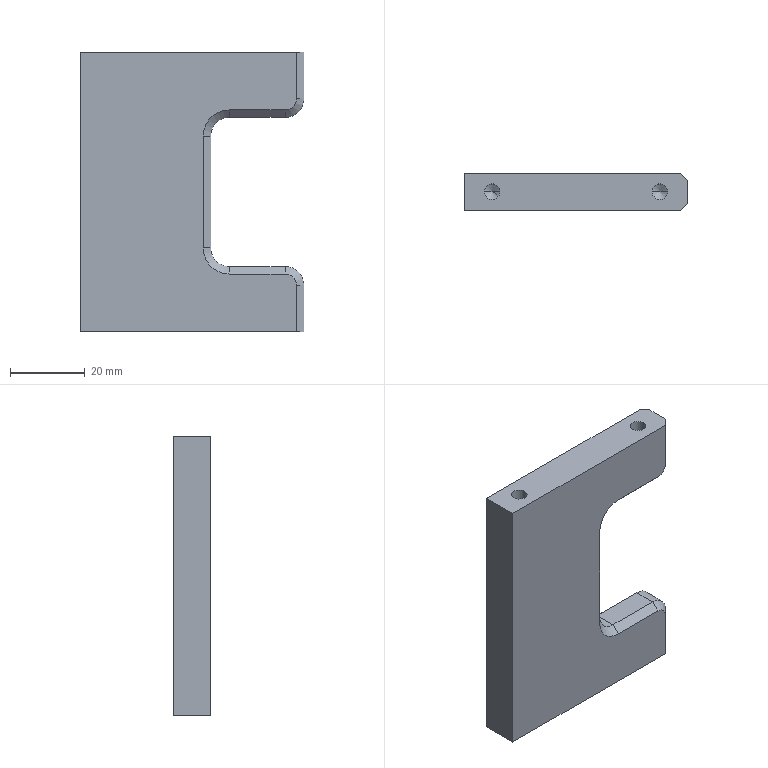Part | SolidWorks | features HoleWzd 2, Chamfer 1, Extrusion 1, Fillet 1, ICE 1 | 1 solid | 48 faces | box 60 x 10 x 75 mm | volume 33824 mm3 | plane 20 | cone 16 | cylinder 12 | commonest cylinder face diameters 4.2 x8 10 x4
STEP:
#1=CARTESIAN_POINT('',(50.4,5.,-12.4));
#2=VERTEX_POINT('',#1);
#3=CARTESIAN_POINT('',(54.6,5.,-12.4));
#4=VERTEX_POINT('',#3);
#5=CARTESIAN_POINT('',(52.5,5.,-12.4));
#6=DIRECTION('',(0.,0.,1.));
#7=DIRECTION('',(1.,0.,0.));
#8=AXIS2_PLACEMENT_3D('',#5,#6,#7);
#9=CIRCLE('',#8,2.1);
#10=EDGE_CURVE('',#2,#4,#9,.T.);
#11=ORIENTED_EDGE('',*,*,#10,.F.);
#12=CARTESIAN_POINT('',(50.4,5.,0.));
#13=VERTEX_POINT('',#12);
#14=CARTESIAN_POINT('',(50.4,5.,0.));
#15=DIRECTION('',(0.,0.,1.));
#16=VECTOR('',#15,1000.);
#17=LINE('',#14,#16);
#18=EDGE_CURVE('',#2,#13,#17,.T.);
#19=ORIENTED_EDGE('',*,*,#18,.T.);
#20=CARTESIAN_POINT('',(54.6,5.,0.));
#21=VERTEX_POINT('',#20);
#22=CARTESIAN_POINT('',(52.5,5.,0.));
#23=DIRECTION('',(0.,0.,1.));
#24=DIRECTION('',(1.,0.,0.));
#25=AXIS2_PLACEMENT_3D('',#22,#23,#24);
#26=CIRCLE('',#25,2.1);
#27=EDGE_CURVE('',#13,#21,#26,.T.);
#28=ORIENTED_EDGE('',*,*,#27,.T.);
#29=CARTESIAN_POINT('',(54.6,5.,0.));
#30=DIRECTION('',(0.,0.,1.));
#31=VECTOR('',#30,1000.);
#32=LINE('',#29,#31);
#33=EDGE_CURVE('',#4,#21,#32,.T.);
#34=ORIENTED_EDGE('',*,*,#33,.F.);
#35=EDGE_LOOP('',(#11,#19,#28,#34));
#36=FACE_OUTER_BOUND('',#35,.T.);
#37=CARTESIAN_POINT('',(52.5,5.,0.));
#38=DIRECTION('',(0.,0.,1.));
#39=DIRECTION('',(1.,0.,0.));
#40=AXIS2_PLACEMENT_3D('',#37,#38,#39);
#41=CYLINDRICAL_SURFACE('',#40,2.1);
#42=ADVANCED_FACE('',(#36),#41,.F.);
#43=CARTESIAN_POINT('',(52.5,5.,-13.662));
#44=VERTEX_POINT('',#43);
#45=CARTESIAN_POINT('',(54.6,5.,-12.4));
#46=DIRECTION('',(0.8572,0.,0.515));
#47=VECTOR('',#46,1000.);
#48=LINE('',#45,#47);
#49=EDGE_CURVE('',#44,#4,#48,.T.);
#50=ORIENTED_EDGE('',*,*,#49,.F.);
#51=CARTESIAN_POINT('',(50.4,5.,-12.4));
#52=DIRECTION('',(-0.8572,0.,0.515));
#53=VECTOR('',#52,1000.);
#54=LINE('',#51,#53);
#55=EDGE_CURVE('',#44,#2,#54,.T.);
#56=ORIENTED_EDGE('',*,*,#55,.T.);
#57=ORIENTED_EDGE('',*,*,#10,.T.);
#58=EDGE_LOOP('',(#50,#56,#57));
#59=FACE_OUTER_BOUND('',#58,.T.);
#60=CARTESIAN_POINT('',(52.5,5.,-12.4));
#61=DIRECTION('',(0.,0.,1.));
#62=DIRECTION('',(1.,0.,0.));
#63=AXIS2_PLACEMENT_3D('',#60,#61,#62);
#64=CONICAL_SURFACE('',#63,2.1,1.03);
#65=ADVANCED_FACE('',(#59),#64,.F.);
#66=CARTESIAN_POINT('',(5.4,5.,-12.4));
#67=VERTEX_POINT('',#66);
#68=CARTESIAN_POINT('',(9.6,5.,-12.4));
#69=VERTEX_POINT('',#68);
#70=CARTESIAN_POINT('',(7.5,5.,-12.4));
#71=DIRECTION('',(0.,0.,1.));
#72=DIRECTION('',(1.,0.,0.));
#73=AXIS2_PLACEMENT_3D('',#70,#71,#72);
#74=CIRCLE('',#73,2.1);
#75=EDGE_CURVE('',#67,#69,#74,.T.);
#76=ORIENTED_EDGE('',*,*,#75,.F.);
#77=CARTESIAN_POINT('',(5.4,5.,0.));
#78=VERTEX_POINT('',#77);
#79=CARTESIAN_POINT('',(5.4,5.,0.));
#80=DIRECTION('',(0.,0.,1.));
#81=VECTOR('',#80,1000.);
#82=LINE('',#79,#81);
#83=EDGE_CURVE('',#67,#78,#82,.T.);
#84=ORIENTED_EDGE('',*,*,#83,.T.);
#85=CARTESIAN_POINT('',(9.6,5.,0.));
#86=VERTEX_POINT('',#85);
#87=CARTESIAN_POINT('',(7.5,5.,0.));
#88=DIRECTION('',(0.,0.,1.));
#89=DIRECTION('',(1.,0.,0.));
#90=AXIS2_PLACEMENT_3D('',#87,#88,#89);
#91=CIRCLE('',#90,2.1);
#92=EDGE_CURVE('',#78,#86,#91,.T.);
#93=ORIENTED_EDGE('',*,*,#92,.T.);
#94=CARTESIAN_POINT('',(9.6,5.,0.));
#95=DIRECTION('',(0.,0.,1.));
#96=VECTOR('',#95,1000.);
#97=LINE('',#94,#96);
#98=EDGE_CURVE('',#69,#86,#97,.T.);
#99=ORIENTED_EDGE('',*,*,#98,.F.);
#100=EDGE_LOOP('',(#76,#84,#93,#99));
#101=FACE_OUTER_BOUND('',#100,.T.);
#102=CARTESIAN_POINT('',(7.5,5.,0.));
#103=DIRECTION('',(0.,0.,1.));
#104=DIRECTION('',(1.,0.,0.));
#105=AXIS2_PLACEMENT_3D('',#102,#103,#104);
#106=CYLINDRICAL_SURFACE('',#105,2.1);
#107=ADVANCED_FACE('',(#101),#106,.F.);
#108=CARTESIAN_POINT('',(7.5,5.,-13.662));
#109=VERTEX_POINT('',#108);
#110=CARTESIAN_POINT('',(9.6,5.,-12.4));
#111=DIRECTION('',(0.8572,0.,0.515));
#112=VECTOR('',#111,1000.);
#113=LINE('',#110,#112);
#114=EDGE_CURVE('',#109,#69,#113,.T.);
#115=ORIENTED_EDGE('',*,*,#114,.F.);
#116=CARTESIAN_POINT('',(5.4,5.,-12.4));
#117=DIRECTION('',(-0.8572,0.,0.515));
#118=VECTOR('',#117,1000.);
#119=LINE('',#116,#118);
#120=EDGE_CURVE('',#109,#67,#119,.T.);
#121=ORIENTED_EDGE('',*,*,#120,.T.);
#122=ORIENTED_EDGE('',*,*,#75,.T.);
#123=EDGE_LOOP('',(#115,#121,#122));
#124=FACE_OUTER_BOUND('',#123,.T.);
#125=CARTESIAN_POINT('',(7.5,5.,-12.4));
#126=DIRECTION('',(0.,0.,1.));
#127=DIRECTION('',(1.,0.,0.));
#128=AXIS2_PLACEMENT_3D('',#125,#126,#127);
#129=CONICAL_SURFACE('',#128,2.1,1.03);
#130=ADVANCED_FACE('',(#124),#129,.F.);
#131=CARTESIAN_POINT('',(9.6,5.,-62.6));
#132=VERTEX_POINT('',#131);
#133=CARTESIAN_POINT('',(5.4,5.,-62.6));
#134=VERTEX_POINT('',#133);
#135=CARTESIAN_POINT('',(7.5,5.,-62.6));
#136=DIRECTION('',(0.,0.,-1.));
#137=DIRECTION('',(-1.,0.,0.));
#138=AXIS2_PLACEMENT_3D('',#135,#136,#137);
#139=CIRCLE('',#138,2.1);
#140=EDGE_CURVE('',#132,#134,#139,.T.);
#141=ORIENTED_EDGE('',*,*,#140,.F.);
#142=CARTESIAN_POINT('',(9.6,5.,-75.));
#143=VERTEX_POINT('',#142);
#144=CARTESIAN_POINT('',(9.6,5.,-75.));
#145=DIRECTION('',(0.,0.,-1.));
#146=VECTOR('',#145,1000.);
#147=LINE('',#144,#146);
#148=EDGE_CURVE('',#132,#143,#147,.T.);
#149=ORIENTED_EDGE('',*,*,#148,.T.);
#150=CARTESIAN_POINT('',(5.4,5.,-75.));
#151=VERTEX_POINT('',#150);
#152=CARTESIAN_POINT('',(7.5,5.,-75.));
#153=DIRECTION('',(0.,0.,-1.));
#154=DIRECTION('',(-1.,0.,0.));
#155=AXIS2_PLACEMENT_3D('',#152,#153,#154);
#156=CIRCLE('',#155,2.1);
#157=EDGE_CURVE('',#143,#151,#156,.T.);
#158=ORIENTED_EDGE('',*,*,#157,.T.);
#159=CARTESIAN_POINT('',(5.4,5.,-75.));
#160=DIRECTION('',(0.,0.,-1.));
#161=VECTOR('',#160,1000.);
#162=LINE('',#159,#161);
#163=EDGE_CURVE('',#134,#151,#162,.T.);
#164=ORIENTED_EDGE('',*,*,#163,.F.);
#165=EDGE_LOOP('',(#141,#149,#158,#164));
#166=FACE_OUTER_BOUND('',#165,.T.);
#167=CARTESIAN_POINT('',(7.5,5.,-75.));
#168=DIRECTION('',(0.,0.,-1.));
#169=DIRECTION('',(-1.,0.,0.));
#170=AXIS2_PLACEMENT_3D('',#167,#168,#169);
#171=CYLINDRICAL_SURFACE('',#170,2.1);
#172=ADVANCED_FACE('',(#166),#171,.F.);
#173=CARTESIAN_POINT('',(7.5,5.,-61.338));
#174=VERTEX_POINT('',#173);
#175=CARTESIAN_POINT('',(5.4,5.,-62.6));
#176=DIRECTION('',(-0.8572,0.,-0.515));
#177=VECTOR('',#176,1000.);
#178=LINE('',#175,#177);
#179=EDGE_CURVE('',#174,#134,#178,.T.);
#180=ORIENTED_EDGE('',*,*,#179,.F.);
#181=CARTESIAN_POINT('',(9.6,5.,-62.6));
#182=DIRECTION('',(0.8572,0.,-0.515));
#183=VECTOR('',#182,1000.);
#184=LINE('',#181,#183);
#185=EDGE_CURVE('',#174,#132,#184,.T.);
#186=ORIENTED_EDGE('',*,*,#185,.T.);
#187=ORIENTED_EDGE('',*,*,#140,.T.);
#188=EDGE_LOOP('',(#180,#186,#187));
#189=FACE_OUTER_BOUND('',#188,.T.);
#190=CARTESIAN_POINT('',(7.5,5.,-62.6));
#191=DIRECTION('',(0.,0.,-1.));
#192=DIRECTION('',(-1.,0.,0.));
#193=AXIS2_PLACEMENT_3D('',#190,#191,#192);
#194=CONICAL_SURFACE('',#193,2.1,1.03);
#195=ADVANCED_FACE('',(#189),#194,.F.);
#196=CARTESIAN_POINT('',(54.6,5.,-62.6));
#197=VERTEX_POINT('',#196);
#198=CARTESIAN_POINT('',(50.4,5.,-62.6));
#199=VERTEX_POINT('',#198);
#200=CARTESIAN_POINT('',(52.5,5.,-62.6));
#201=DIRECTION('',(0.,0.,-1.));
#202=DIRECTION('',(-1.,0.,0.));
#203=AXIS2_PLACEMENT_3D('',#200,#201,#202);
#204=CIRCLE('',#203,2.1);
#205=EDGE_CURVE('',#197,#199,#204,.T.);
#206=ORIENTED_EDGE('',*,*,#205,.F.);
#207=CARTESIAN_POINT('',(54.6,5.,-75.));
#208=VERTEX_POINT('',#207);
#209=CARTESIAN_POINT('',(54.6,5.,-75.));
#210=DIRECTION('',(0.,0.,-1.));
#211=VECTOR('',#210,1000.);
#212=LINE('',#209,#211);
#213=EDGE_CURVE('',#197,#208,#212,.T.);
#214=ORIENTED_EDGE('',*,*,#213,.T.);
#215=CARTESIAN_POINT('',(50.4,5.,-75.));
#216=VERTEX_POINT('',#215);
#217=CARTESIAN_POINT('',(52.5,5.,-75.));
#218=DIRECTION('',(0.,0.,-1.));
#219=DIRECTION('',(-1.,0.,0.));
#220=AXIS2_PLACEMENT_3D('',#217,#218,#219);
#221=CIRCLE('',#220,2.1);
#222=EDGE_CURVE('',#208,#216,#221,.T.);
#223=ORIENTED_EDGE('',*,*,#222,.T.);
#224=CARTESIAN_POINT('',(50.4,5.,-75.));
#225=DIRECTION('',(0.,0.,-1.));
#226=VECTOR('',#225,1000.);
#227=LINE('',#224,#226);
#228=EDGE_CURVE('',#199,#216,#227,.T.);
#229=ORIENTED_EDGE('',*,*,#228,.F.);
#230=EDGE_LOOP('',(#206,#214,#223,#229));
#231=FACE_OUTER_BOUND('',#230,.T.);
#232=CARTESIAN_POINT('',(52.5,5.,-75.));
#233=DIRECTION('',(0.,0.,-1.));
#234=DIRECTION('',(-1.,0.,0.));
#235=AXIS2_PLACEMENT_3D('',#232,#233,#234);
#236=CYLINDRICAL_SURFACE('',#235,2.1);
#237=ADVANCED_FACE('',(#231),#236,.F.);
#238=CARTESIAN_POINT('',(52.5,5.,-61.338));
#239=VERTEX_POINT('',#238);
#240=CARTESIAN_POINT('',(50.4,5.,-62.6));
#241=DIRECTION('',(-0.8572,0.,-0.515));
#242=VECTOR('',#241,1000.);
#243=LINE('',#240,#242);
#244=EDGE_CURVE('',#239,#199,#243,.T.);
#245=ORIENTED_EDGE('',*,*,#244,.F.);
#246=CARTESIAN_POINT('',(54.6,5.,-62.6));
#247=DIRECTION('',(0.8572,0.,-0.515));
#248=VECTOR('',#247,1000.);
#249=LINE('',#246,#248);
#250=EDGE_CURVE('',#239,#197,#249,.T.);
#251=ORIENTED_EDGE('',*,*,#250,.T.);
#252=ORIENTED_EDGE('',*,*,#205,.T.);
#253=EDGE_LOOP('',(#245,#251,#252));
#254=FACE_OUTER_BOUND('',#253,.T.);
#255=CARTESIAN_POINT('',(52.5,5.,-62.6));
#256=DIRECTION('',(0.,0.,-1.));
#257=DIRECTION('',(-1.,0.,0.));
#258=AXIS2_PLACEMENT_3D('',#255,#256,#257);
#259=CONICAL_SURFACE('',#258,2.1,1.03);
#260=ADVANCED_FACE('',(#254),#259,.F.);
#261=CARTESIAN_POINT('',(60.,8.,-62.5));
#262=VERTEX_POINT('',#261);
#263=CARTESIAN_POINT('',(60.,2.,-62.5));
#264=VERTEX_POINT('',#263);
#265=CARTESIAN_POINT('',(60.,10.,-62.5));
#266=DIRECTION('',(0.,-1.,0.));
#267=VECTOR('',#266,1000.);
#268=LINE('',#265,#267);
#269=EDGE_CURVE('',#262,#264,#268,.T.);
#270=ORIENTED_EDGE('',*,*,#269,.T.);
#271=CARTESIAN_POINT('',(60.,2.,-75.));
#272=VERTEX_POINT('',#271);
#273=CARTESIAN_POINT('',(60.,2.,-75.));
#274=DIRECTION('',(0.,0.,-1.));
#275=VECTOR('',#274,1000.);
#276=LINE('',#273,#275);
#277=EDGE_CURVE('',#264,#272,#276,.T.);
#278=ORIENTED_EDGE('',*,*,#277,.T.);
#279=CARTESIAN_POINT('',(60.,8.,-75.));
#280=VERTEX_POINT('',#279);
#281=CARTESIAN_POINT('',(60.,10.,-75.));
#282=DIRECTION('',(0.,-1.,0.));
#283=VECTOR('',#282,1000.);
#284=LINE('',#281,#283);
#285=EDGE_CURVE('',#280,#272,#284,.T.);
#286=ORIENTED_EDGE('',*,*,#285,.F.);
#287=CARTESIAN_POINT('',(60.,8.,0.));
#288=DIRECTION('',(0.,0.,1.));
#289=VECTOR('',#288,1000.);
#290=LINE('',#287,#289);
#291=EDGE_CURVE('',#280,#262,#290,.T.);
#292=ORIENTED_EDGE('',*,*,#291,.T.);
#293=EDGE_LOOP('',(#270,#278,#286,#292));
#294=FACE_OUTER_BOUND('',#293,.T.);
#295=CARTESIAN_POINT('',(60.,10.,0.));
#296=DIRECTION('',(-1.,0.,0.));
#297=DIRECTION('',(0.,0.,1.));
#298=AXIS2_PLACEMENT_3D('',#295,#296,#297);
#299=PLANE('',#298);
#300=ADVANCED_FACE('',(#294),#299,.F.);
#301=CARTESIAN_POINT('',(0.,0.,-75.));
#302=VERTEX_POINT('',#301);
#303=CARTESIAN_POINT('',(0.,0.,0.));
#304=VERTEX_POINT('',#303);
#305=CARTESIAN_POINT('',(0.,0.,0.));
#306=DIRECTION('',(0.,0.,1.));
#307=VECTOR('',#306,1000.);
#308=LINE('',#305,#307);
#309=EDGE_CURVE('',#302,#304,#308,.T.);
#310=ORIENTED_EDGE('',*,*,#309,.T.);
#311=CARTESIAN_POINT('',(0.,10.,0.));
#312=VERTEX_POINT('',#311);
#313=CARTESIAN_POINT('',(0.,10.,0.));
#314=DIRECTION('',(0.,-1.,0.));
#315=VECTOR('',#314,1000.);
#316=LINE('',#313,#315);
#317=EDGE_CURVE('',#312,#304,#316,.T.);
#318=ORIENTED_EDGE('',*,*,#317,.F.);
#319=CARTESIAN_POINT('',(0.,10.,-75.));
#320=VERTEX_POINT('',#319);
#321=CARTESIAN_POINT('',(0.,10.,0.));
#322=DIRECTION('',(0.,0.,1.));
#323=VECTOR('',#322,1000.);
#324=LINE('',#321,#323);
#325=EDGE_CURVE('',#320,#312,#324,.T.);
#326=ORIENTED_EDGE('',*,*,#325,.F.);
#327=CARTESIAN_POINT('',(0.,10.,-75.));
#328=DIRECTION('',(0.,-1.,0.));
#329=VECTOR('',#328,1000.);
#330=LINE('',#327,#329);
#331=EDGE_CURVE('',#320,#302,#330,.T.);
#332=ORIENTED_EDGE('',*,*,#331,.T.);
#333=EDGE_LOOP('',(#310,#318,#326,#332));
#334=FACE_OUTER_BOUND('',#333,.T.);
#335=CARTESIAN_POINT('',(0.,10.,0.));
#336=DIRECTION('',(1.,0.,0.));
#337=DIRECTION('',(0.,0.,-1.));
#338=AXIS2_PLACEMENT_3D('',#335,#336,#337);
#339=PLANE('',#338);
#340=ADVANCED_FACE('',(#334),#339,.F.);
#341=CARTESIAN_POINT('',(52.5,5.,0.));
#342=DIRECTION('',(0.,0.,1.));
#343=DIRECTION('',(1.,0.,0.));
#344=AXIS2_PLACEMENT_3D('',#341,#342,#343);
#345=CIRCLE('',#344,2.1);
#346=EDGE_CURVE('',#21,#13,#345,.T.);
#347=ORIENTED_EDGE('',*,*,#346,.F.);
#348=ORIENTED_EDGE('',*,*,#27,.F.);
#349=EDGE_LOOP('',(#347,#348));
#350=FACE_BOUND('',#349,.T.);
#351=CARTESIAN_POINT('',(7.5,5.,0.));
#352=DIRECTION('',(0.,0.,1.));
#353=DIRECTION('',(1.,0.,0.));
#354=AXIS2_PLACEMENT_3D('',#351,#352,#353);
#355=CIRCLE('',#354,2.1);
#356=EDGE_CURVE('',#86,#78,#355,.T.);
#357=ORIENTED_EDGE('',*,*,#356,.F.);
#358=ORIENTED_EDGE('',*,*,#92,.F.);
#359=EDGE_LOOP('',(#357,#358));
#360=FACE_BOUND('',#359,.T.);
#361=CARTESIAN_POINT('',(58.,0.,0.));
#362=VERTEX_POINT('',#361);
#363=CARTESIAN_POINT('',(0.,0.,0.));
#364=DIRECTION('',(1.,0.,0.));
#365=VECTOR('',#364,1000.);
#366=LINE('',#363,#365);
#367=EDGE_CURVE('',#304,#362,#366,.T.);
#368=ORIENTED_EDGE('',*,*,#367,.T.);
#369=CARTESIAN_POINT('',(60.,2.,0.));
#370=VERTEX_POINT('',#369);
#371=CARTESIAN_POINT('',(60.,2.,0.));
#372=DIRECTION('',(0.7071,0.7071,0.));
#373=VECTOR('',#372,1000.);
#374=LINE('',#371,#373);
#375=EDGE_CURVE('',#362,#370,#374,.T.);
#376=ORIENTED_EDGE('',*,*,#375,.T.);
#377=CARTESIAN_POINT('',(60.,8.,0.));
#378=VERTEX_POINT('',#377);
#379=CARTESIAN_POINT('',(60.,10.,0.));
#380=DIRECTION('',(0.,-1.,0.));
#381=VECTOR('',#380,1000.);
#382=LINE('',#379,#381);
#383=EDGE_CURVE('',#378,#370,#382,.T.);
#384=ORIENTED_EDGE('',*,*,#383,.F.);
#385=CARTESIAN_POINT('',(58.,10.,0.));
#386=VERTEX_POINT('',#385);
#387=CARTESIAN_POINT('',(58.,10.,0.));
#388=DIRECTION('',(-0.7071,0.7071,0.));
#389=VECTOR('',#388,1000.);
#390=LINE('',#387,#389);
#391=EDGE_CURVE('',#378,#386,#390,.T.);
#392=ORIENTED_EDGE('',*,*,#391,.T.);
#393=CARTESIAN_POINT('',(0.,10.,0.));
#394=DIRECTION('',(1.,0.,0.));
#395=VECTOR('',#394,1000.);
#396=LINE('',#393,#395);
#397=EDGE_CURVE('',#312,#386,#396,.T.);
#398=ORIENTED_EDGE('',*,*,#397,.F.);
#399=ORIENTED_EDGE('',*,*,#317,.T.);
#400=EDGE_LOOP('',(#368,#376,#384,#392,#398,#399));
#401=FACE_OUTER_BOUND('',#400,.T.);
#402=CARTESIAN_POINT('',(0.,10.,0.));
#403=DIRECTION('',(0.,0.,-1.));
#404=DIRECTION('',(-1.,0.,0.));
#405=AXIS2_PLACEMENT_3D('',#402,#403,#404);
#406=PLANE('',#405);
#407=ADVANCED_FACE('',(#350,#360,#401),#406,.F.);
#408=ORIENTED_EDGE('',*,*,#383,.T.);
#409=CARTESIAN_POINT('',(60.,2.,-12.5));
#410=VERTEX_POINT('',#409);
#411=CARTESIAN_POINT('',(60.,2.,-12.5));
#412=DIRECTION('',(0.,0.,-1.));
#413=VECTOR('',#412,1000.);
#414=LINE('',#411,#413);
#415=EDGE_CURVE('',#370,#410,#414,.T.);
#416=ORIENTED_EDGE('',*,*,#415,.T.);
#417=CARTESIAN_POINT('',(60.,8.,-12.5));
#418=VERTEX_POINT('',#417);
#419=CARTESIAN_POINT('',(60.,10.,-12.5));
#420=DIRECTION('',(0.,1.,0.));
#421=VECTOR('',#420,1000.);
#422=LINE('',#419,#421);
#423=EDGE_CURVE('',#410,#418,#422,.T.);
#424=ORIENTED_EDGE('',*,*,#423,.T.);
#425=CARTESIAN_POINT('',(60.,8.,0.));
#426=DIRECTION('',(0.,0.,1.));
#427=VECTOR('',#426,1000.);
#428=LINE('',#425,#427);
#429=EDGE_CURVE('',#418,#378,#428,.T.);
#430=ORIENTED_EDGE('',*,*,#429,.T.);
#431=EDGE_LOOP('',(#408,#416,#424,#430));
#432=FACE_OUTER_BOUND('',#431,.T.);
#433=CARTESIAN_POINT('',(60.,10.,0.));
#434=DIRECTION('',(-1.,0.,0.));
#435=DIRECTION('',(0.,0.,1.));
#436=AXIS2_PLACEMENT_3D('',#433,#434,#435);
#437=PLANE('',#436);
#438=ADVANCED_FACE('',(#432),#437,.F.);
#439=CARTESIAN_POINT('',(7.5,5.,-75.));
#440=DIRECTION('',(0.,0.,-1.));
#441=DIRECTION('',(-1.,0.,0.));
#442=AXIS2_PLACEMENT_3D('',#439,#440,#441);
#443=CIRCLE('',#442,2.1);
#444=EDGE_CURVE('',#151,#143,#443,.T.);
#445=ORIENTED_EDGE('',*,*,#444,.F.);
#446=ORIENTED_EDGE('',*,*,#157,.F.);
#447=EDGE_LOOP('',(#445,#446));
#448=FACE_BOUND('',#447,.T.);
#449=CARTESIAN_POINT('',(52.5,5.,-75.));
#450=DIRECTION('',(0.,0.,-1.));
#451=DIRECTION('',(-1.,0.,0.));
#452=AXIS2_PLACEMENT_3D('',#449,#450,#451);
#453=CIRCLE('',#452,2.1);
#454=EDGE_CURVE('',#216,#208,#453,.T.);
#455=ORIENTED_EDGE('',*,*,#454,.F.);
#456=ORIENTED_EDGE('',*,*,#222,.F.);
#457=EDGE_LOOP('',(#455,#456));
#458=FACE_BOUND('',#457,.T.);
#459=ORIENTED_EDGE('',*,*,#285,.T.);
#460=CARTESIAN_POINT('',(58.,0.,-75.));
#461=VERTEX_POINT('',#460);
#462=CARTESIAN_POINT('',(60.,2.,-75.));
#463=DIRECTION('',(-0.7071,-0.7071,0.));
#464=VECTOR('',#463,1000.);
#465=LINE('',#462,#464);
#466=EDGE_CURVE('',#272,#461,#465,.T.);
#467=ORIENTED_EDGE('',*,*,#466,.T.);
#468=CARTESIAN_POINT('',(0.,0.,-75.));
#469=DIRECTION('',(-1.,0.,0.));
#470=VECTOR('',#469,1000.);
#471=LINE('',#468,#470);
#472=EDGE_CURVE('',#461,#302,#471,.T.);
#473=ORIENTED_EDGE('',*,*,#472,.T.);
#474=ORIENTED_EDGE('',*,*,#331,.F.);
#475=CARTESIAN_POINT('',(58.,10.,-75.));
#476=VERTEX_POINT('',#475);
#477=CARTESIAN_POINT('',(0.,10.,-75.));
#478=DIRECTION('',(-1.,0.,0.));
#479=VECTOR('',#478,1000.);
#480=LINE('',#477,#479);
#481=EDGE_CURVE('',#476,#320,#480,.T.);
#482=ORIENTED_EDGE('',*,*,#481,.F.);
#483=CARTESIAN_POINT('',(58.,10.,-75.));
#484=DIRECTION('',(0.7071,-0.7071,0.));
#485=VECTOR('',#484,1000.);
#486=LINE('',#483,#485);
#487=EDGE_CURVE('',#476,#280,#486,.T.);
#488=ORIENTED_EDGE('',*,*,#487,.T.);
#489=EDGE_LOOP('',(#459,#467,#473,#474,#482,#488));
#490=FACE_OUTER_BOUND('',#489,.T.);
#491=CARTESIAN_POINT('',(0.,10.,-75.));
#492=DIRECTION('',(0.,0.,1.));
#493=DIRECTION('',(1.,0.,0.));
#494=AXIS2_PLACEMENT_3D('',#491,#492,#493);
#495=PLANE('',#494);
#496=ADVANCED_FACE('',(#448,#458,#490),#495,.F.);
#497=CARTESIAN_POINT('',(55.,10.,-59.5));
#498=VERTEX_POINT('',#497);
#499=CARTESIAN_POINT('',(58.,10.,-62.5));
#500=VERTEX_POINT('',#499);
#501=CARTESIAN_POINT('',(55.,10.,-62.5));
#502=DIRECTION('',(0.,1.,0.));
#503=DIRECTION('',(0.,0.,-1.));
#504=AXIS2_PLACEMENT_3D('',#501,#502,#503);
#505=CIRCLE('',#504,3.);
#506=EDGE_CURVE('',#498,#500,#505,.T.);
#507=ORIENTED_EDGE('',*,*,#506,.T.);
#508=CARTESIAN_POINT('',(58.,10.,0.));
#509=DIRECTION('',(0.,0.,-1.));
#510=VECTOR('',#509,1000.);
#511=LINE('',#508,#510);
#512=EDGE_CURVE('',#500,#476,#511,.T.);
#513=ORIENTED_EDGE('',*,*,#512,.T.);
#514=ORIENTED_EDGE('',*,*,#481,.T.);
#515=ORIENTED_EDGE('',*,*,#325,.T.);
#516=ORIENTED_EDGE('',*,*,#397,.T.);
#517=CARTESIAN_POINT('',(58.,10.,-12.5));
#518=VERTEX_POINT('',#517);
#519=CARTESIAN_POINT('',(58.,10.,0.));
#520=DIRECTION('',(0.,0.,-1.));
#521=VECTOR('',#520,1000.);
#522=LINE('',#519,#521);
#523=EDGE_CURVE('',#386,#518,#522,.T.);
#524=ORIENTED_EDGE('',*,*,#523,.T.);
#525=CARTESIAN_POINT('',(55.,10.,-15.5));
#526=VERTEX_POINT('',#525);
#527=CARTESIAN_POINT('',(55.,10.,-12.5));
#528=DIRECTION('',(0.,1.,0.));
#529=DIRECTION('',(0.,0.,-1.));
#530=AXIS2_PLACEMENT_3D('',#527,#528,#529);
#531=CIRCLE('',#530,3.);
#532=EDGE_CURVE('',#518,#526,#531,.T.);
#533=ORIENTED_EDGE('',*,*,#532,.T.);
#534=CARTESIAN_POINT('',(40.,10.,-15.5));
#535=VERTEX_POINT('',#534);
#536=CARTESIAN_POINT('',(0.,10.,-15.5));
#537=DIRECTION('',(-1.,0.,0.));
#538=VECTOR('',#537,1000.);
#539=LINE('',#536,#538);
#540=EDGE_CURVE('',#526,#535,#539,.T.);
#541=ORIENTED_EDGE('',*,*,#540,.T.);
#542=CARTESIAN_POINT('',(33.,10.,-22.5));
#543=VERTEX_POINT('',#542);
#544=CARTESIAN_POINT('',(40.,10.,-22.5));
#545=DIRECTION('',(0.,-1.,0.));
#546=DIRECTION('',(0.,0.,-1.));
#547=AXIS2_PLACEMENT_3D('',#544,#545,#546);
#548=CIRCLE('',#547,7.);
#549=EDGE_CURVE('',#535,#543,#548,.T.);
#550=ORIENTED_EDGE('',*,*,#549,.T.);
#551=CARTESIAN_POINT('',(33.,10.,-52.5));
#552=VERTEX_POINT('',#551);
#553=CARTESIAN_POINT('',(33.,10.,0.));
#554=DIRECTION('',(0.,0.,-1.));
#555=VECTOR('',#554,1000.);
#556=LINE('',#553,#555);
#557=EDGE_CURVE('',#543,#552,#556,.T.);
#558=ORIENTED_EDGE('',*,*,#557,.T.);
#559=CARTESIAN_POINT('',(40.,10.,-59.5));
#560=VERTEX_POINT('',#559);
#561=CARTESIAN_POINT('',(40.,10.,-52.5));
#562=DIRECTION('',(0.,-1.,0.));
#563=DIRECTION('',(0.,0.,-1.));
#564=AXIS2_PLACEMENT_3D('',#561,#562,#563);
#565=CIRCLE('',#564,7.);
#566=EDGE_CURVE('',#552,#560,#565,.T.);
#567=ORIENTED_EDGE('',*,*,#566,.T.);
#568=CARTESIAN_POINT('',(0.,10.,-59.5));
#569=DIRECTION('',(1.,0.,0.));
#570=VECTOR('',#569,1000.);
#571=LINE('',#568,#570);
#572=EDGE_CURVE('',#560,#498,#571,.T.);
#573=ORIENTED_EDGE('',*,*,#572,.T.);
#574=EDGE_LOOP('',(#507,#513,#514,#515,#516,#524,#533,#541,#550,#558,#567,#573));
#575=FACE_OUTER_BOUND('',#574,.T.);
#576=CARTESIAN_POINT('',(0.,10.,0.));
#577=DIRECTION('',(0.,-1.,0.));
#578=DIRECTION('',(0.,0.,-1.));
#579=AXIS2_PLACEMENT_3D('',#576,#577,#578);
#580=PLANE('',#579);
#581=ADVANCED_FACE('',(#575),#580,.F.);
#582=ORIENTED_EDGE('',*,*,#472,.F.);
#583=CARTESIAN_POINT('',(58.,0.,-62.5));
#584=VERTEX_POINT('',#583);
#585=CARTESIAN_POINT('',(58.,0.,-62.5));
#586=DIRECTION('',(0.,0.,1.));
#587=VECTOR('',#586,1000.);
#588=LINE('',#585,#587);
#589=EDGE_CURVE('',#461,#584,#588,.T.);
#590=ORIENTED_EDGE('',*,*,#589,.T.);
#591=CARTESIAN_POINT('',(55.,0.,-59.5));
#592=VERTEX_POINT('',#591);
#593=CARTESIAN_POINT('',(55.,0.,-62.5));
#594=DIRECTION('',(0.,-1.,0.));
#595=DIRECTION('',(0.,0.,-1.));
#596=AXIS2_PLACEMENT_3D('',#593,#594,#595);
#597=CIRCLE('',#596,3.);
#598=EDGE_CURVE('',#584,#592,#597,.T.);
#599=ORIENTED_EDGE('',*,*,#598,.T.);
#600=CARTESIAN_POINT('',(40.,0.,-59.5));
#601=VERTEX_POINT('',#600);
#602=CARTESIAN_POINT('',(40.,0.,-59.5));
#603=DIRECTION('',(-1.,0.,0.));
#604=VECTOR('',#603,1000.);
#605=LINE('',#602,#604);
#606=EDGE_CURVE('',#592,#601,#605,.T.);
#607=ORIENTED_EDGE('',*,*,#606,.T.);
#608=CARTESIAN_POINT('',(33.,0.,-52.5));
#609=VERTEX_POINT('',#608);
#610=CARTESIAN_POINT('',(40.,0.,-52.5));
#611=DIRECTION('',(0.,1.,0.));
#612=DIRECTION('',(0.,0.,-1.));
#613=AXIS2_PLACEMENT_3D('',#610,#611,#612);
#614=CIRCLE('',#613,7.);
#615=EDGE_CURVE('',#601,#609,#614,.T.);
#616=ORIENTED_EDGE('',*,*,#615,.T.);
#617=CARTESIAN_POINT('',(33.,0.,-22.5));
#618=VERTEX_POINT('',#617);
#619=CARTESIAN_POINT('',(33.,0.,-22.5));
#620=DIRECTION('',(0.,0.,1.));
#621=VECTOR('',#620,1000.);
#622=LINE('',#619,#621);
#623=EDGE_CURVE('',#609,#618,#622,.T.);
#624=ORIENTED_EDGE('',*,*,#623,.T.);
#625=CARTESIAN_POINT('',(40.,0.,-15.5));
#626=VERTEX_POINT('',#625);
#627=CARTESIAN_POINT('',(40.,0.,-22.5));
#628=DIRECTION('',(0.,1.,0.));
#629=DIRECTION('',(0.,0.,-1.));
#630=AXIS2_PLACEMENT_3D('',#627,#628,#629);
#631=CIRCLE('',#630,7.);
#632=EDGE_CURVE('',#618,#626,#631,.T.);
#633=ORIENTED_EDGE('',*,*,#632,.T.);
#634=CARTESIAN_POINT('',(55.,0.,-15.5));
#635=VERTEX_POINT('',#634);
#636=CARTESIAN_POINT('',(55.,0.,-15.5));
#637=DIRECTION('',(1.,0.,0.));
#638=VECTOR('',#637,1000.);
#639=LINE('',#636,#638);
#640=EDGE_CURVE('',#626,#635,#639,.T.);
#641=ORIENTED_EDGE('',*,*,#640,.T.);
#642=CARTESIAN_POINT('',(58.,0.,-12.5));
#643=VERTEX_POINT('',#642);
#644=CARTESIAN_POINT('',(55.,0.,-12.5));
#645=DIRECTION('',(0.,-1.,0.));
#646=DIRECTION('',(0.,0.,-1.));
#647=AXIS2_PLACEMENT_3D('',#644,#645,#646);
#648=CIRCLE('',#647,3.);
#649=EDGE_CURVE('',#635,#643,#648,.T.);
#650=ORIENTED_EDGE('',*,*,#649,.T.);
#651=CARTESIAN_POINT('',(58.,0.,0.));
#652=DIRECTION('',(0.,0.,1.));
#653=VECTOR('',#652,1000.);
#654=LINE('',#651,#653);
#655=EDGE_CURVE('',#643,#362,#654,.T.);
#656=ORIENTED_EDGE('',*,*,#655,.T.);
#657=ORIENTED_EDGE('',*,*,#367,.F.);
#658=ORIENTED_EDGE('',*,*,#309,.F.);
#659=EDGE_LOOP('',(#582,#590,#599,#607,#616,#624,#633,#641,#650,#656,#657,#658));
#660=FACE_OUTER_BOUND('',#659,.T.);
#661=CARTESIAN_POINT('',(0.,0.,0.));
#662=DIRECTION('',(0.,-1.,0.));
#663=DIRECTION('',(0.,0.,-1.));
#664=AXIS2_PLACEMENT_3D('',#661,#662,#663);
#665=PLANE('',#664);
#666=ADVANCED_FACE('',(#660),#665,.T.);
#667=ORIENTED_EDGE('',*,*,#250,.F.);
#668=ORIENTED_EDGE('',*,*,#244,.T.);
#669=CARTESIAN_POINT('',(52.5,5.,-62.6));
#670=DIRECTION('',(0.,0.,-1.));
#671=DIRECTION('',(-1.,0.,0.));
#672=AXIS2_PLACEMENT_3D('',#669,#670,#671);
#673=CIRCLE('',#672,2.1);
#674=EDGE_CURVE('',#199,#197,#673,.T.);
#675=ORIENTED_EDGE('',*,*,#674,.T.);
#676=EDGE_LOOP('',(#667,#668,#675));
#677=FACE_OUTER_BOUND('',#676,.T.);
#678=CARTESIAN_POINT('',(52.5,5.,-62.6));
#679=DIRECTION('',(0.,0.,-1.));
#680=DIRECTION('',(-1.,0.,0.));
#681=AXIS2_PLACEMENT_3D('',#678,#679,#680);
#682=CONICAL_SURFACE('',#681,2.1,1.03);
#683=ADVANCED_FACE('',(#677),#682,.F.);
#684=ORIENTED_EDGE('',*,*,#213,.F.);
#685=ORIENTED_EDGE('',*,*,#674,.F.);
#686=ORIENTED_EDGE('',*,*,#228,.T.);
#687=ORIENTED_EDGE('',*,*,#454,.T.);
#688=EDGE_LOOP('',(#684,#685,#686,#687));
#689=FACE_OUTER_BOUND('',#688,.T.);
#690=CARTESIAN_POINT('',(52.5,5.,-75.));
#691=DIRECTION('',(0.,0.,-1.));
#692=DIRECTION('',(-1.,0.,0.));
#693=AXIS2_PLACEMENT_3D('',#690,#691,#692);
#694=CYLINDRICAL_SURFACE('',#693,2.1);
#695=ADVANCED_FACE('',(#689),#694,.F.);
#696=ORIENTED_EDGE('',*,*,#185,.F.);
#697=ORIENTED_EDGE('',*,*,#179,.T.);
#698=CARTESIAN_POINT('',(7.5,5.,-62.6));
#699=DIRECTION('',(0.,0.,-1.));
#700=DIRECTION('',(-1.,0.,0.));
#701=AXIS2_PLACEMENT_3D('',#698,#699,#700);
#702=CIRCLE('',#701,2.1);
#703=EDGE_CURVE('',#134,#132,#702,.T.);
#704=ORIENTED_EDGE('',*,*,#703,.T.);
#705=EDGE_LOOP('',(#696,#697,#704));
#706=FACE_OUTER_BOUND('',#705,.T.);
#707=CARTESIAN_POINT('',(7.5,5.,-62.6));
#708=DIRECTION('',(0.,0.,-1.));
#709=DIRECTION('',(-1.,0.,0.));
#710=AXIS2_PLACEMENT_3D('',#707,#708,#709);
#711=CONICAL_SURFACE('',#710,2.1,1.03);
#712=ADVANCED_FACE('',(#706),#711,.F.);
#713=ORIENTED_EDGE('',*,*,#148,.F.);
#714=ORIENTED_EDGE('',*,*,#703,.F.);
#715=ORIENTED_EDGE('',*,*,#163,.T.);
#716=ORIENTED_EDGE('',*,*,#444,.T.);
#717=EDGE_LOOP('',(#713,#714,#715,#716));
#718=FACE_OUTER_BOUND('',#717,.T.);
#719=CARTESIAN_POINT('',(7.5,5.,-75.));
#720=DIRECTION('',(0.,0.,-1.));
#721=DIRECTION('',(-1.,0.,0.));
#722=AXIS2_PLACEMENT_3D('',#719,#720,#721);
#723=CYLINDRICAL_SURFACE('',#722,2.1);
#724=ADVANCED_FACE('',(#718),#723,.F.);
#725=ORIENTED_EDGE('',*,*,#120,.F.);
#726=ORIENTED_EDGE('',*,*,#114,.T.);
#727=CARTESIAN_POINT('',(7.5,5.,-12.4));
#728=DIRECTION('',(0.,0.,1.));
#729=DIRECTION('',(1.,0.,0.));
#730=AXIS2_PLACEMENT_3D('',#727,#728,#729);
#731=CIRCLE('',#730,2.1);
#732=EDGE_CURVE('',#69,#67,#731,.T.);
#733=ORIENTED_EDGE('',*,*,#732,.T.);
#734=EDGE_LOOP('',(#725,#726,#733));
#735=FACE_OUTER_BOUND('',#734,.T.);
#736=CARTESIAN_POINT('',(7.5,5.,-12.4));
#737=DIRECTION('',(0.,0.,1.));
#738=DIRECTION('',(1.,0.,0.));
#739=AXIS2_PLACEMENT_3D('',#736,#737,#738);
#740=CONICAL_SURFACE('',#739,2.1,1.03);
#741=ADVANCED_FACE('',(#735),#740,.F.);
#742=ORIENTED_EDGE('',*,*,#83,.F.);
#743=ORIENTED_EDGE('',*,*,#732,.F.);
#744=ORIENTED_EDGE('',*,*,#98,.T.);
#745=ORIENTED_EDGE('',*,*,#356,.T.);
#746=EDGE_LOOP('',(#742,#743,#744,#745));
#747=FACE_OUTER_BOUND('',#746,.T.);
#748=CARTESIAN_POINT('',(7.5,5.,0.));
#749=DIRECTION('',(0.,0.,1.));
#750=DIRECTION('',(1.,0.,0.));
#751=AXIS2_PLACEMENT_3D('',#748,#749,#750);
#752=CYLINDRICAL_SURFACE('',#751,2.1);
#753=ADVANCED_FACE('',(#747),#752,.F.);
#754=ORIENTED_EDGE('',*,*,#55,.F.);
#755=ORIENTED_EDGE('',*,*,#49,.T.);
#756=CARTESIAN_POINT('',(52.5,5.,-12.4));
#757=DIRECTION('',(0.,0.,1.));
#758=DIRECTION('',(1.,0.,0.));
#759=AXIS2_PLACEMENT_3D('',#756,#757,#758);
#760=CIRCLE('',#759,2.1);
#761=EDGE_CURVE('',#4,#2,#760,.T.);
#762=ORIENTED_EDGE('',*,*,#761,.T.);
#763=EDGE_LOOP('',(#754,#755,#762));
#764=FACE_OUTER_BOUND('',#763,.T.);
#765=CARTESIAN_POINT('',(52.5,5.,-12.4));
#766=DIRECTION('',(0.,0.,1.));
#767=DIRECTION('',(1.,0.,0.));
#768=AXIS2_PLACEMENT_3D('',#765,#766,#767);
#769=CONICAL_SURFACE('',#768,2.1,1.03);
#770=ADVANCED_FACE('',(#764),#769,.F.);
#771=ORIENTED_EDGE('',*,*,#18,.F.);
#772=ORIENTED_EDGE('',*,*,#761,.F.);
#773=ORIENTED_EDGE('',*,*,#33,.T.);
#774=ORIENTED_EDGE('',*,*,#346,.T.);
#775=EDGE_LOOP('',(#771,#772,#773,#774));
#776=FACE_OUTER_BOUND('',#775,.T.);
#777=CARTESIAN_POINT('',(52.5,5.,0.));
#778=DIRECTION('',(0.,0.,1.));
#779=DIRECTION('',(1.,0.,0.));
#780=AXIS2_PLACEMENT_3D('',#777,#778,#779);
#781=CYLINDRICAL_SURFACE('',#780,2.1);
#782=ADVANCED_FACE('',(#776),#781,.F.);
#783=CARTESIAN_POINT('',(35.,8.,-22.5));
#784=VERTEX_POINT('',#783);
#785=CARTESIAN_POINT('',(35.,2.,-22.5));
#786=VERTEX_POINT('',#785);
#787=CARTESIAN_POINT('',(35.,0.,-22.5));
#788=DIRECTION('',(0.,-1.,0.));
#789=VECTOR('',#788,1000.);
#790=LINE('',#787,#789);
#791=EDGE_CURVE('',#784,#786,#790,.T.);
#792=ORIENTED_EDGE('',*,*,#791,.T.);
#793=CARTESIAN_POINT('',(35.,2.,-52.5));
#794=VERTEX_POINT('',#793);
#795=CARTESIAN_POINT('',(35.,2.,-52.5));
#796=DIRECTION('',(0.,0.,-1.));
#797=VECTOR('',#796,1000.);
#798=LINE('',#795,#797);
#799=EDGE_CURVE('',#786,#794,#798,.T.);
#800=ORIENTED_EDGE('',*,*,#799,.T.);
#801=CARTESIAN_POINT('',(35.,8.,-52.5));
#802=VERTEX_POINT('',#801);
#803=CARTESIAN_POINT('',(35.,10.,-52.5));
#804=DIRECTION('',(0.,1.,0.));
#805=VECTOR('',#804,1000.);
#806=LINE('',#803,#805);
#807=EDGE_CURVE('',#794,#802,#806,.T.);
#808=ORIENTED_EDGE('',*,*,#807,.T.);
#809=CARTESIAN_POINT('',(35.,8.,-57.5));
#810=DIRECTION('',(0.,0.,1.));
#811=VECTOR('',#810,1000.);
#812=LINE('',#809,#811);
#813=EDGE_CURVE('',#802,#784,#812,.T.);
#814=ORIENTED_EDGE('',*,*,#813,.T.);
#815=EDGE_LOOP('',(#792,#800,#808,#814));
#816=FACE_OUTER_BOUND('',#815,.T.);
#817=CARTESIAN_POINT('',(35.,0.,-57.5));
#818=DIRECTION('',(-1.,0.,0.));
#819=DIRECTION('',(0.,0.,1.));
#820=AXIS2_PLACEMENT_3D('',#817,#818,#819);
#821=PLANE('',#820);
#822=ADVANCED_FACE('',(#816),#821,.F.);
#823=CARTESIAN_POINT('',(40.,8.,-57.5));
#824=VERTEX_POINT('',#823);
#825=CARTESIAN_POINT('',(40.,2.,-57.5));
#826=VERTEX_POINT('',#825);
#827=CARTESIAN_POINT('',(40.,0.,-57.5));
#828=DIRECTION('',(0.,-1.,0.));
#829=VECTOR('',#828,1000.);
#830=LINE('',#827,#829);
#831=EDGE_CURVE('',#824,#826,#830,.T.);
#832=ORIENTED_EDGE('',*,*,#831,.T.);
#833=CARTESIAN_POINT('',(55.,2.,-57.5));
#834=VERTEX_POINT('',#833);
#835=CARTESIAN_POINT('',(55.,2.,-57.5));
#836=DIRECTION('',(1.,0.,0.));
#837=VECTOR('',#836,1000.);
#838=LINE('',#835,#837);
#839=EDGE_CURVE('',#826,#834,#838,.T.);
#840=ORIENTED_EDGE('',*,*,#839,.T.);
#841=CARTESIAN_POINT('',(55.,8.,-57.5));
#842=VERTEX_POINT('',#841);
#843=CARTESIAN_POINT('',(55.,0.,-57.5));
#844=DIRECTION('',(0.,1.,0.));
#845=VECTOR('',#844,1000.);
#846=LINE('',#843,#845);
#847=EDGE_CURVE('',#834,#842,#846,.T.);
#848=ORIENTED_EDGE('',*,*,#847,.T.);
#849=CARTESIAN_POINT('',(35.,8.,-57.5));
#850=DIRECTION('',(-1.,0.,0.));
#851=VECTOR('',#850,1000.);
#852=LINE('',#849,#851);
#853=EDGE_CURVE('',#842,#824,#852,.T.);
#854=ORIENTED_EDGE('',*,*,#853,.T.);
#855=EDGE_LOOP('',(#832,#840,#848,#854));
#856=FACE_OUTER_BOUND('',#855,.T.);
#857=CARTESIAN_POINT('',(35.,0.,-57.5));
#858=DIRECTION('',(0.,0.,-1.));
#859=DIRECTION('',(-1.,0.,0.));
#860=AXIS2_PLACEMENT_3D('',#857,#858,#859);
#861=PLANE('',#860);
#862=ADVANCED_FACE('',(#856),#861,.F.);
#863=CARTESIAN_POINT('',(55.,8.,-17.5));
#864=VERTEX_POINT('',#863);
#865=CARTESIAN_POINT('',(55.,2.,-17.5));
#866=VERTEX_POINT('',#865);
#867=CARTESIAN_POINT('',(55.,0.,-17.5));
#868=DIRECTION('',(0.,-1.,0.));
#869=VECTOR('',#868,1000.);
#870=LINE('',#867,#869);
#871=EDGE_CURVE('',#864,#866,#870,.T.);
#872=ORIENTED_EDGE('',*,*,#871,.T.);
#873=CARTESIAN_POINT('',(40.,2.,-17.5));
#874=VERTEX_POINT('',#873);
#875=CARTESIAN_POINT('',(40.,2.,-17.5));
#876=DIRECTION('',(-1.,0.,0.));
#877=VECTOR('',#876,1000.);
#878=LINE('',#875,#877);
#879=EDGE_CURVE('',#866,#874,#878,.T.);
#880=ORIENTED_EDGE('',*,*,#879,.T.);
#881=CARTESIAN_POINT('',(40.,8.,-17.5));
#882=VERTEX_POINT('',#881);
#883=CARTESIAN_POINT('',(40.,10.,-17.5));
#884=DIRECTION('',(0.,1.,0.));
#885=VECTOR('',#884,1000.);
#886=LINE('',#883,#885);
#887=EDGE_CURVE('',#874,#882,#886,.T.);
#888=ORIENTED_EDGE('',*,*,#887,.T.);
#889=CARTESIAN_POINT('',(35.,8.,-17.5));
#890=DIRECTION('',(1.,0.,0.));
#891=VECTOR('',#890,1000.);
#892=LINE('',#889,#891);
#893=EDGE_CURVE('',#882,#864,#892,.T.);
#894=ORIENTED_EDGE('',*,*,#893,.T.);
#895=EDGE_LOOP('',(#872,#880,#888,#894));
#896=FACE_OUTER_BOUND('',#895,.T.);
#897=CARTESIAN_POINT('',(35.,0.,-17.5));
#898=DIRECTION('',(0.,0.,1.));
#899=DIRECTION('',(1.,0.,0.));
#900=AXIS2_PLACEMENT_3D('',#897,#898,#899);
#901=PLANE('',#900);
#902=ADVANCED_FACE('',(#896),#901,.F.);
#903=ORIENTED_EDGE('',*,*,#847,.F.);
#904=CARTESIAN_POINT('',(55.,2.,-62.5));
#905=DIRECTION('',(0.,1.,0.));
#906=DIRECTION('',(0.,0.,-1.));
#907=AXIS2_PLACEMENT_3D('',#904,#905,#906);
#908=CIRCLE('',#907,5.);
#909=EDGE_CURVE('',#834,#264,#908,.T.);
#910=ORIENTED_EDGE('',*,*,#909,.T.);
#911=ORIENTED_EDGE('',*,*,#269,.F.);
#912=CARTESIAN_POINT('',(55.,8.,-62.5));
#913=DIRECTION('',(0.,-1.,0.));
#914=DIRECTION('',(0.,0.,-1.));
#915=AXIS2_PLACEMENT_3D('',#912,#913,#914);
#916=CIRCLE('',#915,5.);
#917=EDGE_CURVE('',#262,#842,#916,.T.);
#918=ORIENTED_EDGE('',*,*,#917,.T.);
#919=EDGE_LOOP('',(#903,#910,#911,#918));
#920=FACE_OUTER_BOUND('',#919,.T.);
#921=CARTESIAN_POINT('',(55.,0.,-62.5));
#922=DIRECTION('',(0.,1.,0.));
#923=DIRECTION('',(0.,0.,1.));
#924=AXIS2_PLACEMENT_3D('',#921,#922,#923);
#925=CYLINDRICAL_SURFACE('',#924,5.);
#926=ADVANCED_FACE('',(#920),#925,.T.);
#927=ORIENTED_EDGE('',*,*,#423,.F.);
#928=CARTESIAN_POINT('',(55.,2.,-12.5));
#929=DIRECTION('',(0.,1.,0.));
#930=DIRECTION('',(0.,0.,-1.));
#931=AXIS2_PLACEMENT_3D('',#928,#929,#930);
#932=CIRCLE('',#931,5.);
#933=EDGE_CURVE('',#410,#866,#932,.T.);
#934=ORIENTED_EDGE('',*,*,#933,.T.);
#935=ORIENTED_EDGE('',*,*,#871,.F.);
#936=CARTESIAN_POINT('',(55.,8.,-12.5));
#937=DIRECTION('',(0.,-1.,0.));
#938=DIRECTION('',(0.,0.,-1.));
#939=AXIS2_PLACEMENT_3D('',#936,#937,#938);
#940=CIRCLE('',#939,5.);
#941=EDGE_CURVE('',#864,#418,#940,.T.);
#942=ORIENTED_EDGE('',*,*,#941,.T.);
#943=EDGE_LOOP('',(#927,#934,#935,#942));
#944=FACE_OUTER_BOUND('',#943,.T.);
#945=CARTESIAN_POINT('',(55.,10.,-12.5));
#946=DIRECTION('',(0.,1.,0.));
#947=DIRECTION('',(0.,0.,1.));
#948=AXIS2_PLACEMENT_3D('',#945,#946,#947);
#949=CYLINDRICAL_SURFACE('',#948,5.);
#950=ADVANCED_FACE('',(#944),#949,.T.);
#951=ORIENTED_EDGE('',*,*,#887,.F.);
#952=CARTESIAN_POINT('',(40.,2.,-22.5));
#953=DIRECTION('',(0.,-1.,0.));
#954=DIRECTION('',(0.,0.,-1.));
#955=AXIS2_PLACEMENT_3D('',#952,#953,#954);
#956=CIRCLE('',#955,5.);
#957=EDGE_CURVE('',#874,#786,#956,.T.);
#958=ORIENTED_EDGE('',*,*,#957,.T.);
#959=ORIENTED_EDGE('',*,*,#791,.F.);
#960=CARTESIAN_POINT('',(40.,8.,-22.5));
#961=DIRECTION('',(0.,1.,0.));
#962=DIRECTION('',(0.,0.,-1.));
#963=AXIS2_PLACEMENT_3D('',#960,#961,#962);
#964=CIRCLE('',#963,5.);
#965=EDGE_CURVE('',#784,#882,#964,.T.);
#966=ORIENTED_EDGE('',*,*,#965,.T.);
#967=EDGE_LOOP('',(#951,#958,#959,#966));
#968=FACE_OUTER_BOUND('',#967,.T.);
#969=CARTESIAN_POINT('',(40.,0.,-22.5));
#970=DIRECTION('',(0.,-1.,0.));
#971=DIRECTION('',(0.,0.,-1.));
#972=AXIS2_PLACEMENT_3D('',#969,#970,#971);
#973=CYLINDRICAL_SURFACE('',#972,5.);
#974=ADVANCED_FACE('',(#968),#973,.F.);
#975=ORIENTED_EDGE('',*,*,#807,.F.);
#976=CARTESIAN_POINT('',(40.,2.,-52.5));
#977=DIRECTION('',(0.,-1.,0.));
#978=DIRECTION('',(0.,0.,-1.));
#979=AXIS2_PLACEMENT_3D('',#976,#977,#978);
#980=CIRCLE('',#979,5.);
#981=EDGE_CURVE('',#794,#826,#980,.T.);
#982=ORIENTED_EDGE('',*,*,#981,.T.);
#983=ORIENTED_EDGE('',*,*,#831,.F.);
#984=CARTESIAN_POINT('',(40.,8.,-52.5));
#985=DIRECTION('',(0.,1.,0.));
#986=DIRECTION('',(0.,0.,-1.));
#987=AXIS2_PLACEMENT_3D('',#984,#985,#986);
#988=CIRCLE('',#987,5.);
#989=EDGE_CURVE('',#824,#802,#988,.T.);
#990=ORIENTED_EDGE('',*,*,#989,.T.);
#991=EDGE_LOOP('',(#975,#982,#983,#990));
#992=FACE_OUTER_BOUND('',#991,.T.);
#993=CARTESIAN_POINT('',(40.,0.,-52.5));
#994=DIRECTION('',(0.,-1.,0.));
#995=DIRECTION('',(0.,0.,-1.));
#996=AXIS2_PLACEMENT_3D('',#993,#994,#995);
#997=CYLINDRICAL_SURFACE('',#996,5.);
#998=ADVANCED_FACE('',(#992),#997,.F.);
#999=ORIENTED_EDGE('',*,*,#375,.F.);
#1000=ORIENTED_EDGE('',*,*,#655,.F.);
#1001=CARTESIAN_POINT('',(60.,2.,-12.5));
#1002=DIRECTION('',(-0.7071,-0.7071,0.));
#1003=VECTOR('',#1002,1000.);
#1004=LINE('',#1001,#1003);
#1005=EDGE_CURVE('',#410,#643,#1004,.T.);
#1006=ORIENTED_EDGE('',*,*,#1005,.F.);
#1007=ORIENTED_EDGE('',*,*,#415,.F.);
#1008=EDGE_LOOP('',(#999,#1000,#1006,#1007));
#1009=FACE_OUTER_BOUND('',#1008,.T.);
#1010=CARTESIAN_POINT('',(60.,2.,0.));
#1011=DIRECTION('',(0.7071,-0.7071,0.));
#1012=DIRECTION('',(0.,0.,1.));
#1013=AXIS2_PLACEMENT_3D('',#1010,#1011,#1012);
#1014=PLANE('',#1013);
#1015=ADVANCED_FACE('',(#1009),#1014,.T.);
#1016=ORIENTED_EDGE('',*,*,#1005,.T.);
#1017=ORIENTED_EDGE('',*,*,#649,.F.);
#1018=CARTESIAN_POINT('',(55.,2.,-17.5));
#1019=DIRECTION('',(0.,-0.7071,0.7071));
#1020=VECTOR('',#1019,1000.);
#1021=LINE('',#1018,#1020);
#1022=EDGE_CURVE('',#866,#635,#1021,.T.);
#1023=ORIENTED_EDGE('',*,*,#1022,.F.);
#1024=ORIENTED_EDGE('',*,*,#933,.F.);
#1025=EDGE_LOOP('',(#1016,#1017,#1023,#1024));
#1026=FACE_OUTER_BOUND('',#1025,.T.);
#1027=CARTESIAN_POINT('',(55.,0.,-12.5));
#1028=DIRECTION('',(0.,1.,0.));
#1029=DIRECTION('',(0.,0.,1.));
#1030=AXIS2_PLACEMENT_3D('',#1027,#1028,#1029);
#1031=CONICAL_SURFACE('',#1030,3.,0.7854);
#1032=ADVANCED_FACE('',(#1026),#1031,.T.);
#1033=ORIENTED_EDGE('',*,*,#1022,.T.);
#1034=ORIENTED_EDGE('',*,*,#640,.F.);
#1035=CARTESIAN_POINT('',(40.,2.,-17.5));
#1036=DIRECTION('',(0.,-0.7071,0.7071));
#1037=VECTOR('',#1036,1000.);
#1038=LINE('',#1035,#1037);
#1039=EDGE_CURVE('',#874,#626,#1038,.T.);
#1040=ORIENTED_EDGE('',*,*,#1039,.F.);
#1041=ORIENTED_EDGE('',*,*,#879,.F.);
#1042=EDGE_LOOP('',(#1033,#1034,#1040,#1041));
#1043=FACE_OUTER_BOUND('',#1042,.T.);
#1044=CARTESIAN_POINT('',(0.,0.,-15.5));
#1045=DIRECTION('',(0.,-0.7071,-0.7071));
#1046=DIRECTION('',(-1.,0.,0.));
#1047=AXIS2_PLACEMENT_3D('',#1044,#1045,#1046);
#1048=PLANE('',#1047);
#1049=ADVANCED_FACE('',(#1043),#1048,.T.);
#1050=ORIENTED_EDGE('',*,*,#1039,.T.);
#1051=ORIENTED_EDGE('',*,*,#632,.F.);
#1052=CARTESIAN_POINT('',(35.,2.,-22.5));
#1053=DIRECTION('',(-0.7071,-0.7071,0.));
#1054=VECTOR('',#1053,1000.);
#1055=LINE('',#1052,#1054);
#1056=EDGE_CURVE('',#786,#618,#1055,.T.);
#1057=ORIENTED_EDGE('',*,*,#1056,.F.);
#1058=ORIENTED_EDGE('',*,*,#957,.F.);
#1059=EDGE_LOOP('',(#1050,#1051,#1057,#1058));
#1060=FACE_OUTER_BOUND('',#1059,.T.);
#1061=CARTESIAN_POINT('',(40.,0.,-22.5));
#1062=DIRECTION('',(0.,-1.,0.));
#1063=DIRECTION('',(0.,0.,-1.));
#1064=AXIS2_PLACEMENT_3D('',#1061,#1062,#1063);
#1065=CONICAL_SURFACE('',#1064,7.,0.7854);
#1066=ADVANCED_FACE('',(#1060),#1065,.F.);
#1067=ORIENTED_EDGE('',*,*,#1056,.T.);
#1068=ORIENTED_EDGE('',*,*,#623,.F.);
#1069=CARTESIAN_POINT('',(35.,2.,-52.5));
#1070=DIRECTION('',(-0.7071,-0.7071,0.));
#1071=VECTOR('',#1070,1000.);
#1072=LINE('',#1069,#1071);
#1073=EDGE_CURVE('',#794,#609,#1072,.T.);
#1074=ORIENTED_EDGE('',*,*,#1073,.F.);
#1075=ORIENTED_EDGE('',*,*,#799,.F.);
#1076=EDGE_LOOP('',(#1067,#1068,#1074,#1075));
#1077=FACE_OUTER_BOUND('',#1076,.T.);
#1078=CARTESIAN_POINT('',(33.,0.,0.));
#1079=DIRECTION('',(0.7071,-0.7071,0.));
#1080=DIRECTION('',(0.,0.,-1.));
#1081=AXIS2_PLACEMENT_3D('',#1078,#1079,#1080);
#1082=PLANE('',#1081);
#1083=ADVANCED_FACE('',(#1077),#1082,.T.);
#1084=ORIENTED_EDGE('',*,*,#1073,.T.);
#1085=ORIENTED_EDGE('',*,*,#615,.F.);
#1086=CARTESIAN_POINT('',(40.,2.,-57.5));
#1087=DIRECTION('',(0.,-0.7071,-0.7071));
#1088=VECTOR('',#1087,1000.);
#1089=LINE('',#1086,#1088);
#1090=EDGE_CURVE('',#826,#601,#1089,.T.);
#1091=ORIENTED_EDGE('',*,*,#1090,.F.);
#1092=ORIENTED_EDGE('',*,*,#981,.F.);
#1093=EDGE_LOOP('',(#1084,#1085,#1091,#1092));
#1094=FACE_OUTER_BOUND('',#1093,.T.);
#1095=CARTESIAN_POINT('',(40.,0.,-52.5));
#1096=DIRECTION('',(0.,-1.,0.));
#1097=DIRECTION('',(0.,0.,-1.));
#1098=AXIS2_PLACEMENT_3D('',#1095,#1096,#1097);
#1099=CONICAL_SURFACE('',#1098,7.,0.7854);
#1100=ADVANCED_FACE('',(#1094),#1099,.F.);
#1101=ORIENTED_EDGE('',*,*,#1090,.T.);
#1102=ORIENTED_EDGE('',*,*,#606,.F.);
#1103=CARTESIAN_POINT('',(55.,2.,-57.5));
#1104=DIRECTION('',(0.,-0.7071,-0.7071));
#1105=VECTOR('',#1104,1000.);
#1106=LINE('',#1103,#1105);
#1107=EDGE_CURVE('',#834,#592,#1106,.T.);
#1108=ORIENTED_EDGE('',*,*,#1107,.F.);
#1109=ORIENTED_EDGE('',*,*,#839,.F.);
#1110=EDGE_LOOP('',(#1101,#1102,#1108,#1109));
#1111=FACE_OUTER_BOUND('',#1110,.T.);
#1112=CARTESIAN_POINT('',(0.,0.,-59.5));
#1113=DIRECTION('',(0.,-0.7071,0.7071));
#1114=DIRECTION('',(1.,0.,0.));
#1115=AXIS2_PLACEMENT_3D('',#1112,#1113,#1114);
#1116=PLANE('',#1115);
#1117=ADVANCED_FACE('',(#1111),#1116,.T.);
#1118=ORIENTED_EDGE('',*,*,#1107,.T.);
#1119=ORIENTED_EDGE('',*,*,#598,.F.);
#1120=CARTESIAN_POINT('',(60.,2.,-62.5));
#1121=DIRECTION('',(-0.7071,-0.7071,0.));
#1122=VECTOR('',#1121,1000.);
#1123=LINE('',#1120,#1122);
#1124=EDGE_CURVE('',#264,#584,#1123,.T.);
#1125=ORIENTED_EDGE('',*,*,#1124,.F.);
#1126=ORIENTED_EDGE('',*,*,#909,.F.);
#1127=EDGE_LOOP('',(#1118,#1119,#1125,#1126));
#1128=FACE_OUTER_BOUND('',#1127,.T.);
#1129=CARTESIAN_POINT('',(55.,0.,-62.5));
#1130=DIRECTION('',(0.,1.,0.));
#1131=DIRECTION('',(0.,0.,1.));
#1132=AXIS2_PLACEMENT_3D('',#1129,#1130,#1131);
#1133=CONICAL_SURFACE('',#1132,3.,0.7854);
#1134=ADVANCED_FACE('',(#1128),#1133,.T.);
#1135=ORIENTED_EDGE('',*,*,#1124,.T.);
#1136=ORIENTED_EDGE('',*,*,#589,.F.);
#1137=ORIENTED_EDGE('',*,*,#466,.F.);
#1138=ORIENTED_EDGE('',*,*,#277,.F.);
#1139=EDGE_LOOP('',(#1135,#1136,#1137,#1138));
#1140=FACE_OUTER_BOUND('',#1139,.T.);
#1141=CARTESIAN_POINT('',(60.,2.,0.));
#1142=DIRECTION('',(0.7071,-0.7071,0.));
#1143=DIRECTION('',(0.,0.,1.));
#1144=AXIS2_PLACEMENT_3D('',#1141,#1142,#1143);
#1145=PLANE('',#1144);
#1146=ADVANCED_FACE('',(#1140),#1145,.T.);
#1147=ORIENTED_EDGE('',*,*,#391,.F.);
#1148=ORIENTED_EDGE('',*,*,#429,.F.);
#1149=CARTESIAN_POINT('',(58.,10.,-12.5));
#1150=DIRECTION('',(0.7071,-0.7071,0.));
#1151=VECTOR('',#1150,1000.);
#1152=LINE('',#1149,#1151);
#1153=EDGE_CURVE('',#518,#418,#1152,.T.);
#1154=ORIENTED_EDGE('',*,*,#1153,.F.);
#1155=ORIENTED_EDGE('',*,*,#523,.F.);
#1156=EDGE_LOOP('',(#1147,#1148,#1154,#1155));
#1157=FACE_OUTER_BOUND('',#1156,.T.);
#1158=CARTESIAN_POINT('',(58.,10.,0.));
#1159=DIRECTION('',(-0.7071,-0.7071,0.));
#1160=DIRECTION('',(0.,0.,-1.));
#1161=AXIS2_PLACEMENT_3D('',#1158,#1159,#1160);
#1162=PLANE('',#1161);
#1163=ADVANCED_FACE('',(#1157),#1162,.F.);
#1164=ORIENTED_EDGE('',*,*,#1153,.T.);
#1165=ORIENTED_EDGE('',*,*,#941,.F.);
#1166=CARTESIAN_POINT('',(55.,10.,-15.5));
#1167=DIRECTION('',(0.,-0.7071,-0.7071));
#1168=VECTOR('',#1167,1000.);
#1169=LINE('',#1166,#1168);
#1170=EDGE_CURVE('',#526,#864,#1169,.T.);
#1171=ORIENTED_EDGE('',*,*,#1170,.F.);
#1172=ORIENTED_EDGE('',*,*,#532,.F.);
#1173=EDGE_LOOP('',(#1164,#1165,#1171,#1172));
#1174=FACE_OUTER_BOUND('',#1173,.T.);
#1175=CARTESIAN_POINT('',(55.,10.,-12.5));
#1176=DIRECTION('',(0.,-1.,0.));
#1177=DIRECTION('',(0.,0.,-1.));
#1178=AXIS2_PLACEMENT_3D('',#1175,#1176,#1177);
#1179=CONICAL_SURFACE('',#1178,3.,0.7854);
#1180=ADVANCED_FACE('',(#1174),#1179,.T.);
#1181=ORIENTED_EDGE('',*,*,#1170,.T.);
#1182=ORIENTED_EDGE('',*,*,#893,.F.);
#1183=CARTESIAN_POINT('',(40.,10.,-15.5));
#1184=DIRECTION('',(0.,-0.7071,-0.7071));
#1185=VECTOR('',#1184,1000.);
#1186=LINE('',#1183,#1185);
#1187=EDGE_CURVE('',#535,#882,#1186,.T.);
#1188=ORIENTED_EDGE('',*,*,#1187,.F.);
#1189=ORIENTED_EDGE('',*,*,#540,.F.);
#1190=EDGE_LOOP('',(#1181,#1182,#1188,#1189));
#1191=FACE_OUTER_BOUND('',#1190,.T.);
#1192=CARTESIAN_POINT('',(35.,8.,-17.5));
#1193=DIRECTION('',(0.,-0.7071,0.7071));
#1194=DIRECTION('',(1.,0.,0.));
#1195=AXIS2_PLACEMENT_3D('',#1192,#1193,#1194);
#1196=PLANE('',#1195);
#1197=ADVANCED_FACE('',(#1191),#1196,.F.);
#1198=ORIENTED_EDGE('',*,*,#1187,.T.);
#1199=ORIENTED_EDGE('',*,*,#965,.F.);
#1200=CARTESIAN_POINT('',(33.,10.,-22.5));
#1201=DIRECTION('',(0.7071,-0.7071,0.));
#1202=VECTOR('',#1201,1000.);
#1203=LINE('',#1200,#1202);
#1204=EDGE_CURVE('',#543,#784,#1203,.T.);
#1205=ORIENTED_EDGE('',*,*,#1204,.F.);
#1206=ORIENTED_EDGE('',*,*,#549,.F.);
#1207=EDGE_LOOP('',(#1198,#1199,#1205,#1206));
#1208=FACE_OUTER_BOUND('',#1207,.T.);
#1209=CARTESIAN_POINT('',(40.,10.,-22.5));
#1210=DIRECTION('',(0.,1.,0.));
#1211=DIRECTION('',(0.,0.,1.));
#1212=AXIS2_PLACEMENT_3D('',#1209,#1210,#1211);
#1213=CONICAL_SURFACE('',#1212,7.,0.7854);
#1214=ADVANCED_FACE('',(#1208),#1213,.F.);
#1215=ORIENTED_EDGE('',*,*,#1204,.T.);
#1216=ORIENTED_EDGE('',*,*,#813,.F.);
#1217=CARTESIAN_POINT('',(33.,10.,-52.5));
#1218=DIRECTION('',(0.7071,-0.7071,0.));
#1219=VECTOR('',#1218,1000.);
#1220=LINE('',#1217,#1219);
#1221=EDGE_CURVE('',#552,#802,#1220,.T.);
#1222=ORIENTED_EDGE('',*,*,#1221,.F.);
#1223=ORIENTED_EDGE('',*,*,#557,.F.);
#1224=EDGE_LOOP('',(#1215,#1216,#1222,#1223));
#1225=FACE_OUTER_BOUND('',#1224,.T.);
#1226=CARTESIAN_POINT('',(35.,8.,-57.5));
#1227=DIRECTION('',(-0.7071,-0.7071,0.));
#1228=DIRECTION('',(0.,0.,1.));
#1229=AXIS2_PLACEMENT_3D('',#1226,#1227,#1228);
#1230=PLANE('',#1229);
#1231=ADVANCED_FACE('',(#1225),#1230,.F.);
#1232=ORIENTED_EDGE('',*,*,#1221,.T.);
#1233=ORIENTED_EDGE('',*,*,#989,.F.);
#1234=CARTESIAN_POINT('',(40.,10.,-59.5));
#1235=DIRECTION('',(0.,-0.7071,0.7071));
#1236=VECTOR('',#1235,1000.);
#1237=LINE('',#1234,#1236);
#1238=EDGE_CURVE('',#560,#824,#1237,.T.);
#1239=ORIENTED_EDGE('',*,*,#1238,.F.);
#1240=ORIENTED_EDGE('',*,*,#566,.F.);
#1241=EDGE_LOOP('',(#1232,#1233,#1239,#1240));
#1242=FACE_OUTER_BOUND('',#1241,.T.);
#1243=CARTESIAN_POINT('',(40.,10.,-52.5));
#1244=DIRECTION('',(0.,1.,0.));
#1245=DIRECTION('',(0.,0.,1.));
#1246=AXIS2_PLACEMENT_3D('',#1243,#1244,#1245);
#1247=CONICAL_SURFACE('',#1246,7.,0.7854);
#1248=ADVANCED_FACE('',(#1242),#1247,.F.);
#1249=ORIENTED_EDGE('',*,*,#1238,.T.);
#1250=ORIENTED_EDGE('',*,*,#853,.F.);
#1251=CARTESIAN_POINT('',(55.,10.,-59.5));
#1252=DIRECTION('',(0.,-0.7071,0.7071));
#1253=VECTOR('',#1252,1000.);
#1254=LINE('',#1251,#1253);
#1255=EDGE_CURVE('',#498,#842,#1254,.T.);
#1256=ORIENTED_EDGE('',*,*,#1255,.F.);
#1257=ORIENTED_EDGE('',*,*,#572,.F.);
#1258=EDGE_LOOP('',(#1249,#1250,#1256,#1257));
#1259=FACE_OUTER_BOUND('',#1258,.T.);
#1260=CARTESIAN_POINT('',(35.,8.,-57.5));
#1261=DIRECTION('',(0.,-0.7071,-0.7071));
#1262=DIRECTION('',(-1.,0.,0.));
#1263=AXIS2_PLACEMENT_3D('',#1260,#1261,#1262);
#1264=PLANE('',#1263);
#1265=ADVANCED_FACE('',(#1259),#1264,.F.);
#1266=ORIENTED_EDGE('',*,*,#1255,.T.);
#1267=ORIENTED_EDGE('',*,*,#917,.F.);
#1268=CARTESIAN_POINT('',(58.,10.,-62.5));
#1269=DIRECTION('',(0.7071,-0.7071,0.));
#1270=VECTOR('',#1269,1000.);
#1271=LINE('',#1268,#1270);
#1272=EDGE_CURVE('',#500,#262,#1271,.T.);
#1273=ORIENTED_EDGE('',*,*,#1272,.F.);
#1274=ORIENTED_EDGE('',*,*,#506,.F.);
#1275=EDGE_LOOP('',(#1266,#1267,#1273,#1274));
#1276=FACE_OUTER_BOUND('',#1275,.T.);
#1277=CARTESIAN_POINT('',(55.,10.,-62.5));
#1278=DIRECTION('',(0.,-1.,0.));
#1279=DIRECTION('',(0.,0.,-1.));
#1280=AXIS2_PLACEMENT_3D('',#1277,#1278,#1279);
#1281=CONICAL_SURFACE('',#1280,3.,0.7854);
#1282=ADVANCED_FACE('',(#1276),#1281,.T.);
#1283=ORIENTED_EDGE('',*,*,#1272,.T.);
#1284=ORIENTED_EDGE('',*,*,#291,.F.);
#1285=ORIENTED_EDGE('',*,*,#487,.F.);
#1286=ORIENTED_EDGE('',*,*,#512,.F.);
#1287=EDGE_LOOP('',(#1283,#1284,#1285,#1286));
#1288=FACE_OUTER_BOUND('',#1287,.T.);
#1289=CARTESIAN_POINT('',(58.,10.,0.));
#1290=DIRECTION('',(-0.7071,-0.7071,0.));
#1291=DIRECTION('',(0.,0.,-1.));
#1292=AXIS2_PLACEMENT_3D('',#1289,#1290,#1291);
#1293=PLANE('',#1292);
#1294=ADVANCED_FACE('',(#1288),#1293,.F.);
#1295=CLOSED_SHELL('',(#42,#65,#107,#130,#172,#195,#237,#260,#300,#340,#407,#438,#496,#581,#666,#683,#695,#712,#724,#741,#753,#770,#782,#822,#862,#902,#926,#950,#974,#998,#1015,#1032,#1049,#1066,#1083,#1100,#1117,#1134,#1146,#1163,#1180,#1197,#1214,#1231,#1248,#1265,#1282,#1294));
#1296=MANIFOLD_SOLID_BREP('',#1295);
#1297=CARTESIAN_POINT('',(0.,0.,0.));
#1298=DIRECTION('',(0.,0.,1.));
#1299=DIRECTION('',(1.,0.,0.));
#1300=AXIS2_PLACEMENT_3D('',#1297,#1298,#1299);
#1301=(LENGTH_UNIT()NAMED_UNIT(*)SI_UNIT(.MILLI.,.METRE.));
#1302=UNCERTAINTY_MEASURE_WITH_UNIT(LENGTH_MEASURE(0.00001),#1301,'','');
#1303=(NAMED_UNIT(*)PLANE_ANGLE_UNIT()SI_UNIT($,.RADIAN.));
#1304=(NAMED_UNIT(*)SI_UNIT($,.STERADIAN.)SOLID_ANGLE_UNIT());
#1305=(GEOMETRIC_REPRESENTATION_CONTEXT(3)GLOBAL_UNCERTAINTY_ASSIGNED_CONTEXT((#1302))GLOBAL_UNIT_ASSIGNED_CONTEXT((#1301,#1303,#1304))REPRESENTATION_CONTEXT('',''));
#1306=ADVANCED_BREP_SHAPE_REPRESENTATION('',(#1296,#1300),#1305);